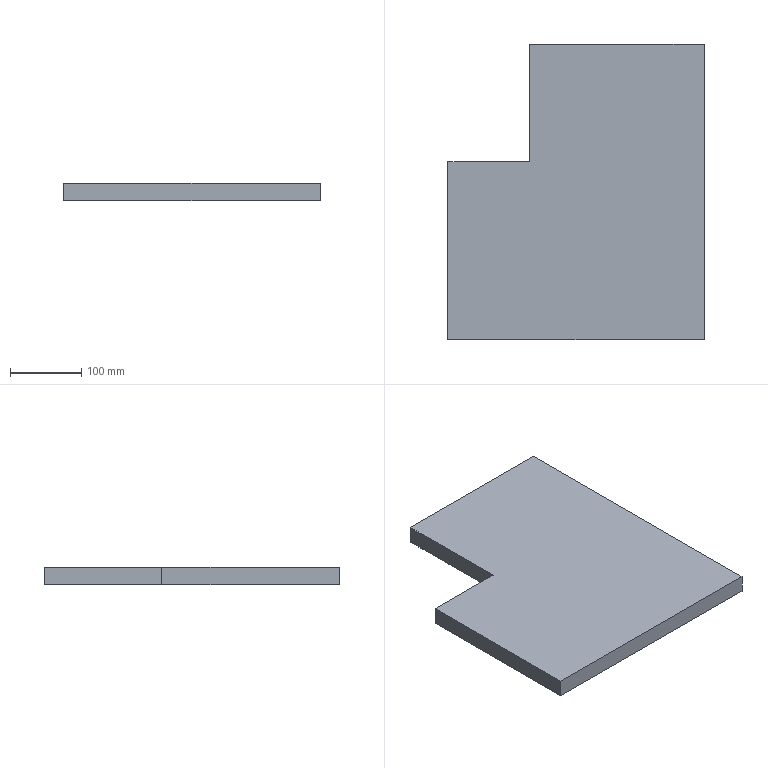Part | SolidWorks | features Extrusion 1 | 1 solid | 8 faces | box 360 x 415 x 25 mm | volume 3260625 mm3 | plane 8
STEP:
#1=CARTESIAN_POINT('',(0.,0.,0.));
#2=VERTEX_POINT('',#1);
#3=CARTESIAN_POINT('',(-245.,0.,0.));
#4=VERTEX_POINT('',#3);
#5=CARTESIAN_POINT('',(0.,0.,0.));
#6=DIRECTION('',(-1.,0.,0.));
#7=VECTOR('',#6,1000.);
#8=LINE('',#5,#7);
#9=EDGE_CURVE('',#2,#4,#8,.T.);
#10=ORIENTED_EDGE('',*,*,#9,.T.);
#11=CARTESIAN_POINT('',(-245.,0.,25.));
#12=VERTEX_POINT('',#11);
#13=CARTESIAN_POINT('',(-245.,0.,25.));
#14=DIRECTION('',(0.,0.,-1.));
#15=VECTOR('',#14,1000.);
#16=LINE('',#13,#15);
#17=EDGE_CURVE('',#12,#4,#16,.T.);
#18=ORIENTED_EDGE('',*,*,#17,.F.);
#19=CARTESIAN_POINT('',(0.,0.,25.));
#20=VERTEX_POINT('',#19);
#21=CARTESIAN_POINT('',(0.,0.,25.));
#22=DIRECTION('',(-1.,0.,0.));
#23=VECTOR('',#22,1000.);
#24=LINE('',#21,#23);
#25=EDGE_CURVE('',#20,#12,#24,.T.);
#26=ORIENTED_EDGE('',*,*,#25,.F.);
#27=CARTESIAN_POINT('',(0.,0.,25.));
#28=DIRECTION('',(0.,0.,-1.));
#29=VECTOR('',#28,1000.);
#30=LINE('',#27,#29);
#31=EDGE_CURVE('',#20,#2,#30,.T.);
#32=ORIENTED_EDGE('',*,*,#31,.T.);
#33=EDGE_LOOP('',(#10,#18,#26,#32));
#34=FACE_OUTER_BOUND('',#33,.T.);
#35=CARTESIAN_POINT('',(0.,0.,25.));
#36=DIRECTION('',(0.,-1.,0.));
#37=DIRECTION('',(0.,0.,-1.));
#38=AXIS2_PLACEMENT_3D('',#35,#36,#37);
#39=PLANE('',#38);
#40=ADVANCED_FACE('',(#34),#39,.F.);
#41=CARTESIAN_POINT('',(-245.,-165.,0.));
#42=VERTEX_POINT('',#41);
#43=CARTESIAN_POINT('',(-245.,0.,0.));
#44=DIRECTION('',(0.,-1.,0.));
#45=VECTOR('',#44,1000.);
#46=LINE('',#43,#45);
#47=EDGE_CURVE('',#4,#42,#46,.T.);
#48=ORIENTED_EDGE('',*,*,#47,.T.);
#49=CARTESIAN_POINT('',(-245.,-165.,25.));
#50=VERTEX_POINT('',#49);
#51=CARTESIAN_POINT('',(-245.,-165.,25.));
#52=DIRECTION('',(0.,0.,-1.));
#53=VECTOR('',#52,1000.);
#54=LINE('',#51,#53);
#55=EDGE_CURVE('',#50,#42,#54,.T.);
#56=ORIENTED_EDGE('',*,*,#55,.F.);
#57=CARTESIAN_POINT('',(-245.,0.,25.));
#58=DIRECTION('',(0.,-1.,0.));
#59=VECTOR('',#58,1000.);
#60=LINE('',#57,#59);
#61=EDGE_CURVE('',#12,#50,#60,.T.);
#62=ORIENTED_EDGE('',*,*,#61,.F.);
#63=ORIENTED_EDGE('',*,*,#17,.T.);
#64=EDGE_LOOP('',(#48,#56,#62,#63));
#65=FACE_OUTER_BOUND('',#64,.T.);
#66=CARTESIAN_POINT('',(-245.,0.,25.));
#67=DIRECTION('',(1.,0.,0.));
#68=DIRECTION('',(0.,1.,0.));
#69=AXIS2_PLACEMENT_3D('',#66,#67,#68);
#70=PLANE('',#69);
#71=ADVANCED_FACE('',(#65),#70,.F.);
#72=CARTESIAN_POINT('',(-360.,-165.,0.));
#73=VERTEX_POINT('',#72);
#74=CARTESIAN_POINT('',(-245.,-165.,0.));
#75=DIRECTION('',(-1.,0.,0.));
#76=VECTOR('',#75,1000.);
#77=LINE('',#74,#76);
#78=EDGE_CURVE('',#42,#73,#77,.T.);
#79=ORIENTED_EDGE('',*,*,#78,.T.);
#80=CARTESIAN_POINT('',(-360.,-165.,25.));
#81=VERTEX_POINT('',#80);
#82=CARTESIAN_POINT('',(-360.,-165.,25.));
#83=DIRECTION('',(0.,0.,-1.));
#84=VECTOR('',#83,1000.);
#85=LINE('',#82,#84);
#86=EDGE_CURVE('',#81,#73,#85,.T.);
#87=ORIENTED_EDGE('',*,*,#86,.F.);
#88=CARTESIAN_POINT('',(-245.,-165.,25.));
#89=DIRECTION('',(-1.,0.,0.));
#90=VECTOR('',#89,1000.);
#91=LINE('',#88,#90);
#92=EDGE_CURVE('',#50,#81,#91,.T.);
#93=ORIENTED_EDGE('',*,*,#92,.F.);
#94=ORIENTED_EDGE('',*,*,#55,.T.);
#95=EDGE_LOOP('',(#79,#87,#93,#94));
#96=FACE_OUTER_BOUND('',#95,.T.);
#97=CARTESIAN_POINT('',(-245.,-165.,25.));
#98=DIRECTION('',(0.,-1.,0.));
#99=DIRECTION('',(1.,0.,0.));
#100=AXIS2_PLACEMENT_3D('',#97,#98,#99);
#101=PLANE('',#100);
#102=ADVANCED_FACE('',(#96),#101,.F.);
#103=CARTESIAN_POINT('',(-360.,-415.,0.));
#104=VERTEX_POINT('',#103);
#105=CARTESIAN_POINT('',(-360.,-165.,0.));
#106=DIRECTION('',(0.,-1.,0.));
#107=VECTOR('',#106,1000.);
#108=LINE('',#105,#107);
#109=EDGE_CURVE('',#73,#104,#108,.T.);
#110=ORIENTED_EDGE('',*,*,#109,.T.);
#111=CARTESIAN_POINT('',(-360.,-415.,25.));
#112=VERTEX_POINT('',#111);
#113=CARTESIAN_POINT('',(-360.,-415.,25.));
#114=DIRECTION('',(0.,0.,-1.));
#115=VECTOR('',#114,1000.);
#116=LINE('',#113,#115);
#117=EDGE_CURVE('',#112,#104,#116,.T.);
#118=ORIENTED_EDGE('',*,*,#117,.F.);
#119=CARTESIAN_POINT('',(-360.,-165.,25.));
#120=DIRECTION('',(0.,-1.,0.));
#121=VECTOR('',#120,1000.);
#122=LINE('',#119,#121);
#123=EDGE_CURVE('',#81,#112,#122,.T.);
#124=ORIENTED_EDGE('',*,*,#123,.F.);
#125=ORIENTED_EDGE('',*,*,#86,.T.);
#126=EDGE_LOOP('',(#110,#118,#124,#125));
#127=FACE_OUTER_BOUND('',#126,.T.);
#128=CARTESIAN_POINT('',(-360.,-165.,25.));
#129=DIRECTION('',(1.,0.,0.));
#130=DIRECTION('',(0.,1.,0.));
#131=AXIS2_PLACEMENT_3D('',#128,#129,#130);
#132=PLANE('',#131);
#133=ADVANCED_FACE('',(#127),#132,.F.);
#134=CARTESIAN_POINT('',(0.,-415.,0.));
#135=VERTEX_POINT('',#134);
#136=CARTESIAN_POINT('',(0.,-415.,0.));
#137=DIRECTION('',(1.,0.,0.));
#138=VECTOR('',#137,1000.);
#139=LINE('',#136,#138);
#140=EDGE_CURVE('',#104,#135,#139,.T.);
#141=ORIENTED_EDGE('',*,*,#140,.T.);
#142=CARTESIAN_POINT('',(0.,-415.,25.));
#143=VERTEX_POINT('',#142);
#144=CARTESIAN_POINT('',(0.,-415.,25.));
#145=DIRECTION('',(0.,0.,-1.));
#146=VECTOR('',#145,1000.);
#147=LINE('',#144,#146);
#148=EDGE_CURVE('',#143,#135,#147,.T.);
#149=ORIENTED_EDGE('',*,*,#148,.F.);
#150=CARTESIAN_POINT('',(0.,-415.,25.));
#151=DIRECTION('',(1.,0.,0.));
#152=VECTOR('',#151,1000.);
#153=LINE('',#150,#152);
#154=EDGE_CURVE('',#112,#143,#153,.T.);
#155=ORIENTED_EDGE('',*,*,#154,.F.);
#156=ORIENTED_EDGE('',*,*,#117,.T.);
#157=EDGE_LOOP('',(#141,#149,#155,#156));
#158=FACE_OUTER_BOUND('',#157,.T.);
#159=CARTESIAN_POINT('',(0.,-415.,25.));
#160=DIRECTION('',(0.,1.,0.));
#161=DIRECTION('',(-1.,0.,0.));
#162=AXIS2_PLACEMENT_3D('',#159,#160,#161);
#163=PLANE('',#162);
#164=ADVANCED_FACE('',(#158),#163,.F.);
#165=CARTESIAN_POINT('',(0.,0.,0.));
#166=DIRECTION('',(0.,1.,0.));
#167=VECTOR('',#166,1000.);
#168=LINE('',#165,#167);
#169=EDGE_CURVE('',#135,#2,#168,.T.);
#170=ORIENTED_EDGE('',*,*,#169,.T.);
#171=ORIENTED_EDGE('',*,*,#31,.F.);
#172=CARTESIAN_POINT('',(0.,0.,25.));
#173=DIRECTION('',(0.,1.,0.));
#174=VECTOR('',#173,1000.);
#175=LINE('',#172,#174);
#176=EDGE_CURVE('',#143,#20,#175,.T.);
#177=ORIENTED_EDGE('',*,*,#176,.F.);
#178=ORIENTED_EDGE('',*,*,#148,.T.);
#179=EDGE_LOOP('',(#170,#171,#177,#178));
#180=FACE_OUTER_BOUND('',#179,.T.);
#181=CARTESIAN_POINT('',(0.,0.,25.));
#182=DIRECTION('',(-1.,0.,0.));
#183=DIRECTION('',(0.,-1.,0.));
#184=AXIS2_PLACEMENT_3D('',#181,#182,#183);
#185=PLANE('',#184);
#186=ADVANCED_FACE('',(#180),#185,.F.);
#187=ORIENTED_EDGE('',*,*,#25,.T.);
#188=ORIENTED_EDGE('',*,*,#61,.T.);
#189=ORIENTED_EDGE('',*,*,#92,.T.);
#190=ORIENTED_EDGE('',*,*,#123,.T.);
#191=ORIENTED_EDGE('',*,*,#154,.T.);
#192=ORIENTED_EDGE('',*,*,#176,.T.);
#193=EDGE_LOOP('',(#187,#188,#189,#190,#191,#192));
#194=FACE_OUTER_BOUND('',#193,.T.);
#195=CARTESIAN_POINT('',(0.,0.,25.));
#196=DIRECTION('',(0.,0.,1.));
#197=DIRECTION('',(1.,0.,0.));
#198=AXIS2_PLACEMENT_3D('',#195,#196,#197);
#199=PLANE('',#198);
#200=ADVANCED_FACE('',(#194),#199,.T.);
#201=ORIENTED_EDGE('',*,*,#9,.F.);
#202=ORIENTED_EDGE('',*,*,#169,.F.);
#203=ORIENTED_EDGE('',*,*,#140,.F.);
#204=ORIENTED_EDGE('',*,*,#109,.F.);
#205=ORIENTED_EDGE('',*,*,#78,.F.);
#206=ORIENTED_EDGE('',*,*,#47,.F.);
#207=EDGE_LOOP('',(#201,#202,#203,#204,#205,#206));
#208=FACE_OUTER_BOUND('',#207,.T.);
#209=CARTESIAN_POINT('',(0.,0.,0.));
#210=DIRECTION('',(0.,0.,1.));
#211=DIRECTION('',(1.,0.,0.));
#212=AXIS2_PLACEMENT_3D('',#209,#210,#211);
#213=PLANE('',#212);
#214=ADVANCED_FACE('',(#208),#213,.F.);
#215=CLOSED_SHELL('',(#40,#71,#102,#133,#164,#186,#200,#214));
#216=MANIFOLD_SOLID_BREP('',#215);
#217=CARTESIAN_POINT('',(0.,0.,0.));
#218=DIRECTION('',(0.,0.,1.));
#219=DIRECTION('',(1.,0.,0.));
#220=AXIS2_PLACEMENT_3D('',#217,#218,#219);
#221=(LENGTH_UNIT()NAMED_UNIT(*)SI_UNIT(.MILLI.,.METRE.));
#222=UNCERTAINTY_MEASURE_WITH_UNIT(LENGTH_MEASURE(0.00001),#221,'','');
#223=(NAMED_UNIT(*)PLANE_ANGLE_UNIT()SI_UNIT($,.RADIAN.));
#224=(NAMED_UNIT(*)SI_UNIT($,.STERADIAN.)SOLID_ANGLE_UNIT());
#225=(GEOMETRIC_REPRESENTATION_CONTEXT(3)GLOBAL_UNCERTAINTY_ASSIGNED_CONTEXT((#222))GLOBAL_UNIT_ASSIGNED_CONTEXT((#221,#223,#224))REPRESENTATION_CONTEXT('',''));
#226=ADVANCED_BREP_SHAPE_REPRESENTATION('',(#216,#220),#225);